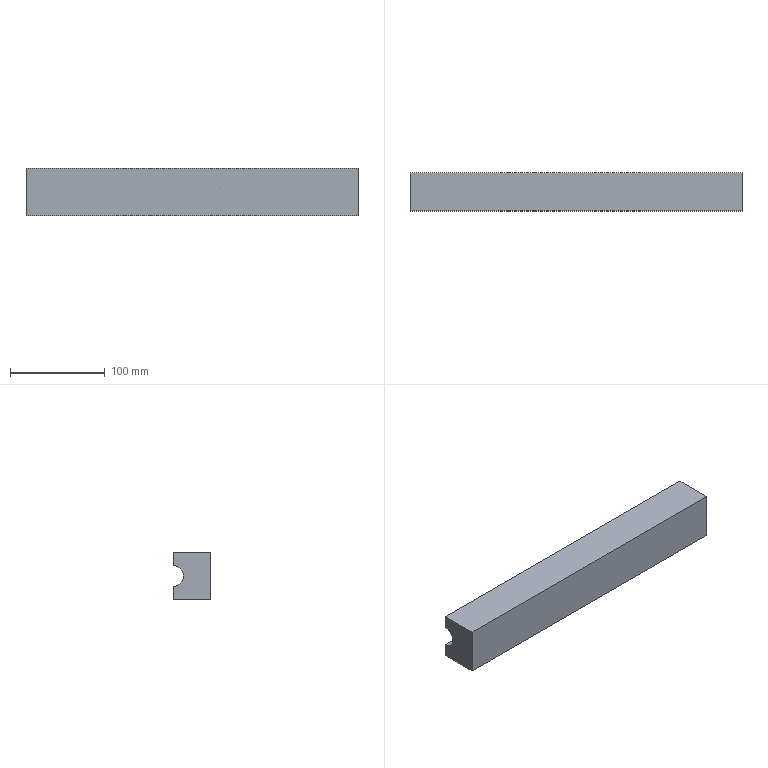Part | NX | features upper clamp 2 | 1 solid | 8 faces | box 350 x 40 x 50 mm | volume 632262 mm3 | plane 7 | cylinder 1 | commonest cylinder face diameters 22.2 x1
STEP:
#1=CARTESIAN_POINT('',(0.,0.,-11.1));
#2=VERTEX_POINT('',#1);
#3=CARTESIAN_POINT('',(0.,0.,11.1));
#4=VERTEX_POINT('',#3);
#5=CARTESIAN_POINT('',(0.,0.,0.));
#6=DIRECTION('',(1.,0.,0.));
#7=DIRECTION('',(0.,1.,0.));
#8=AXIS2_PLACEMENT_3D('',#5,#6,#7);
#9=CIRCLE('',#8,11.1);
#10=EDGE_CURVE('',#2,#4,#9,.F.);
#11=ORIENTED_EDGE('',*,*,#10,.F.);
#12=CARTESIAN_POINT('',(-350.,0.,-11.1));
#13=VERTEX_POINT('',#12);
#14=CARTESIAN_POINT('',(0.,0.,-11.1));
#15=DIRECTION('',(-1.,0.,0.));
#16=VECTOR('',#15,1000.);
#17=LINE('',#14,#16);
#18=EDGE_CURVE('',#13,#2,#17,.F.);
#19=ORIENTED_EDGE('',*,*,#18,.F.);
#20=CARTESIAN_POINT('',(-350.,0.,11.1));
#21=VERTEX_POINT('',#20);
#22=CARTESIAN_POINT('',(-350.,0.,0.));
#23=DIRECTION('',(1.,0.,0.));
#24=DIRECTION('',(0.,1.,0.));
#25=AXIS2_PLACEMENT_3D('',#22,#23,#24);
#26=CIRCLE('',#25,11.1);
#27=EDGE_CURVE('',#21,#13,#26,.T.);
#28=ORIENTED_EDGE('',*,*,#27,.F.);
#29=CARTESIAN_POINT('',(0.,0.,11.1));
#30=DIRECTION('',(-1.,0.,0.));
#31=VECTOR('',#30,1000.);
#32=LINE('',#29,#31);
#33=EDGE_CURVE('',#4,#21,#32,.T.);
#34=ORIENTED_EDGE('',*,*,#33,.F.);
#35=EDGE_LOOP('',(#11,#19,#28,#34));
#36=FACE_BOUND('',#35,.T.);
#37=CARTESIAN_POINT('',(-350.,0.,0.));
#38=DIRECTION('',(1.,0.,0.));
#39=DIRECTION('',(0.,1.,0.));
#40=AXIS2_PLACEMENT_3D('',#37,#38,#39);
#41=CYLINDRICAL_SURFACE('',#40,11.1);
#42=ADVANCED_FACE('',(#36),#41,.F.);
#43=CARTESIAN_POINT('',(-350.,0.,25.));
#44=VERTEX_POINT('',#43);
#45=CARTESIAN_POINT('',(0.,0.,25.));
#46=VERTEX_POINT('',#45);
#47=CARTESIAN_POINT('',(0.,0.,25.));
#48=DIRECTION('',(-1.,0.,0.));
#49=VECTOR('',#48,1000.);
#50=LINE('',#47,#49);
#51=EDGE_CURVE('',#44,#46,#50,.F.);
#52=ORIENTED_EDGE('',*,*,#51,.T.);
#53=CARTESIAN_POINT('',(0.,0.,-25.));
#54=DIRECTION('',(0.,0.,-1.));
#55=VECTOR('',#54,1000.);
#56=LINE('',#53,#55);
#57=EDGE_CURVE('',#4,#46,#56,.F.);
#58=ORIENTED_EDGE('',*,*,#57,.F.);
#59=ORIENTED_EDGE('',*,*,#33,.T.);
#60=CARTESIAN_POINT('',(-350.,0.,-25.));
#61=DIRECTION('',(0.,0.,1.));
#62=VECTOR('',#61,1000.);
#63=LINE('',#60,#62);
#64=EDGE_CURVE('',#44,#21,#63,.F.);
#65=ORIENTED_EDGE('',*,*,#64,.F.);
#66=EDGE_LOOP('',(#52,#58,#59,#65));
#67=FACE_BOUND('',#66,.T.);
#68=CARTESIAN_POINT('',(0.,0.,-25.));
#69=DIRECTION('',(0.,1.,0.));
#70=DIRECTION('',(-1.,0.,0.));
#71=AXIS2_PLACEMENT_3D('',#68,#69,#70);
#72=PLANE('',#71);
#73=ADVANCED_FACE('',(#67),#72,.T.);
#74=CARTESIAN_POINT('',(-350.,0.,-25.));
#75=VERTEX_POINT('',#74);
#76=CARTESIAN_POINT('',(0.,0.,-25.));
#77=VERTEX_POINT('',#76);
#78=CARTESIAN_POINT('',(0.,0.,-25.));
#79=DIRECTION('',(-1.,0.,0.));
#80=VECTOR('',#79,1000.);
#81=LINE('',#78,#80);
#82=EDGE_CURVE('',#75,#77,#81,.F.);
#83=ORIENTED_EDGE('',*,*,#82,.F.);
#84=CARTESIAN_POINT('',(-350.,0.,-25.));
#85=DIRECTION('',(0.,0.,1.));
#86=VECTOR('',#85,1000.);
#87=LINE('',#84,#86);
#88=EDGE_CURVE('',#13,#75,#87,.F.);
#89=ORIENTED_EDGE('',*,*,#88,.F.);
#90=ORIENTED_EDGE('',*,*,#18,.T.);
#91=CARTESIAN_POINT('',(0.,0.,-25.));
#92=DIRECTION('',(0.,0.,-1.));
#93=VECTOR('',#92,1000.);
#94=LINE('',#91,#93);
#95=EDGE_CURVE('',#77,#2,#94,.F.);
#96=ORIENTED_EDGE('',*,*,#95,.F.);
#97=EDGE_LOOP('',(#83,#89,#90,#96));
#98=FACE_BOUND('',#97,.T.);
#99=CARTESIAN_POINT('',(0.,0.,-25.));
#100=DIRECTION('',(0.,1.,0.));
#101=DIRECTION('',(-1.,0.,0.));
#102=AXIS2_PLACEMENT_3D('',#99,#100,#101);
#103=PLANE('',#102);
#104=ADVANCED_FACE('',(#98),#103,.T.);
#105=ORIENTED_EDGE('',*,*,#51,.F.);
#106=CARTESIAN_POINT('',(-350.,-40.,25.));
#107=VERTEX_POINT('',#106);
#108=CARTESIAN_POINT('',(-350.,0.,25.));
#109=DIRECTION('',(0.,1.,0.));
#110=VECTOR('',#109,1000.);
#111=LINE('',#108,#110);
#112=EDGE_CURVE('',#107,#44,#111,.T.);
#113=ORIENTED_EDGE('',*,*,#112,.F.);
#114=CARTESIAN_POINT('',(0.,-40.,25.));
#115=VERTEX_POINT('',#114);
#116=CARTESIAN_POINT('',(0.,-40.,25.));
#117=DIRECTION('',(1.,0.,0.));
#118=VECTOR('',#117,1000.);
#119=LINE('',#116,#118);
#120=EDGE_CURVE('',#115,#107,#119,.F.);
#121=ORIENTED_EDGE('',*,*,#120,.F.);
#122=CARTESIAN_POINT('',(0.,0.,25.));
#123=DIRECTION('',(0.,1.,0.));
#124=VECTOR('',#123,1000.);
#125=LINE('',#122,#124);
#126=EDGE_CURVE('',#46,#115,#125,.F.);
#127=ORIENTED_EDGE('',*,*,#126,.F.);
#128=EDGE_LOOP('',(#105,#113,#121,#127));
#129=FACE_BOUND('',#128,.T.);
#130=CARTESIAN_POINT('',(0.,-40.,25.));
#131=DIRECTION('',(0.,0.,-1.));
#132=DIRECTION('',(-1.,0.,0.));
#133=AXIS2_PLACEMENT_3D('',#130,#131,#132);
#134=PLANE('',#133);
#135=ADVANCED_FACE('',(#129),#134,.F.);
#136=ORIENTED_EDGE('',*,*,#112,.T.);
#137=ORIENTED_EDGE('',*,*,#64,.T.);
#138=ORIENTED_EDGE('',*,*,#27,.T.);
#139=ORIENTED_EDGE('',*,*,#88,.T.);
#140=CARTESIAN_POINT('',(-350.,-40.,-25.));
#141=VERTEX_POINT('',#140);
#142=CARTESIAN_POINT('',(-350.,-40.,-25.));
#143=DIRECTION('',(0.,1.,0.));
#144=VECTOR('',#143,1000.);
#145=LINE('',#142,#144);
#146=EDGE_CURVE('',#141,#75,#145,.T.);
#147=ORIENTED_EDGE('',*,*,#146,.F.);
#148=CARTESIAN_POINT('',(-350.,-40.,-25.));
#149=DIRECTION('',(0.,0.,1.));
#150=VECTOR('',#149,1000.);
#151=LINE('',#148,#150);
#152=EDGE_CURVE('',#107,#141,#151,.F.);
#153=ORIENTED_EDGE('',*,*,#152,.F.);
#154=EDGE_LOOP('',(#136,#137,#138,#139,#147,#153));
#155=FACE_BOUND('',#154,.T.);
#156=CARTESIAN_POINT('',(-350.,0.,-25.));
#157=DIRECTION('',(-1.,0.,0.));
#158=DIRECTION('',(0.,0.,1.));
#159=AXIS2_PLACEMENT_3D('',#156,#157,#158);
#160=PLANE('',#159);
#161=ADVANCED_FACE('',(#155),#160,.T.);
#162=ORIENTED_EDGE('',*,*,#146,.T.);
#163=ORIENTED_EDGE('',*,*,#82,.T.);
#164=CARTESIAN_POINT('',(0.,-40.,-25.));
#165=VERTEX_POINT('',#164);
#166=CARTESIAN_POINT('',(0.,0.,-25.));
#167=DIRECTION('',(0.,1.,0.));
#168=VECTOR('',#167,1000.);
#169=LINE('',#166,#168);
#170=EDGE_CURVE('',#165,#77,#169,.T.);
#171=ORIENTED_EDGE('',*,*,#170,.F.);
#172=CARTESIAN_POINT('',(0.,-40.,-25.));
#173=DIRECTION('',(1.,0.,0.));
#174=VECTOR('',#173,1000.);
#175=LINE('',#172,#174);
#176=EDGE_CURVE('',#141,#165,#175,.T.);
#177=ORIENTED_EDGE('',*,*,#176,.F.);
#178=EDGE_LOOP('',(#162,#163,#171,#177));
#179=FACE_BOUND('',#178,.T.);
#180=CARTESIAN_POINT('',(0.,-40.,-25.));
#181=DIRECTION('',(0.,0.,-1.));
#182=DIRECTION('',(-1.,0.,0.));
#183=AXIS2_PLACEMENT_3D('',#180,#181,#182);
#184=PLANE('',#183);
#185=ADVANCED_FACE('',(#179),#184,.T.);
#186=ORIENTED_EDGE('',*,*,#170,.T.);
#187=ORIENTED_EDGE('',*,*,#95,.T.);
#188=ORIENTED_EDGE('',*,*,#10,.T.);
#189=ORIENTED_EDGE('',*,*,#57,.T.);
#190=ORIENTED_EDGE('',*,*,#126,.T.);
#191=CARTESIAN_POINT('',(0.,-40.,-25.));
#192=DIRECTION('',(0.,0.,1.));
#193=VECTOR('',#192,1000.);
#194=LINE('',#191,#193);
#195=EDGE_CURVE('',#165,#115,#194,.T.);
#196=ORIENTED_EDGE('',*,*,#195,.F.);
#197=EDGE_LOOP('',(#186,#187,#188,#189,#190,#196));
#198=FACE_BOUND('',#197,.T.);
#199=CARTESIAN_POINT('',(0.,0.,-25.));
#200=DIRECTION('',(1.,0.,0.));
#201=DIRECTION('',(0.,0.,-1.));
#202=AXIS2_PLACEMENT_3D('',#199,#200,#201);
#203=PLANE('',#202);
#204=ADVANCED_FACE('',(#198),#203,.T.);
#205=ORIENTED_EDGE('',*,*,#176,.T.);
#206=ORIENTED_EDGE('',*,*,#195,.T.);
#207=ORIENTED_EDGE('',*,*,#120,.T.);
#208=ORIENTED_EDGE('',*,*,#152,.T.);
#209=EDGE_LOOP('',(#205,#206,#207,#208));
#210=FACE_BOUND('',#209,.T.);
#211=CARTESIAN_POINT('',(0.,-40.,-25.));
#212=DIRECTION('',(0.,-1.,0.));
#213=DIRECTION('',(1.,0.,0.));
#214=AXIS2_PLACEMENT_3D('',#211,#212,#213);
#215=PLANE('',#214);
#216=ADVANCED_FACE('',(#210),#215,.T.);
#217=CLOSED_SHELL('',(#42,#73,#104,#135,#161,#185,#204,#216));
#218=MANIFOLD_SOLID_BREP('',#217);
#219=(LENGTH_UNIT()NAMED_UNIT(*)SI_UNIT(.MILLI.,.METRE.));
#220=UNCERTAINTY_MEASURE_WITH_UNIT(LENGTH_MEASURE(0.00001),#219,'','');
#221=(NAMED_UNIT(*)PLANE_ANGLE_UNIT()SI_UNIT($,.RADIAN.));
#222=(NAMED_UNIT(*)SI_UNIT($,.STERADIAN.)SOLID_ANGLE_UNIT());
#223=(GEOMETRIC_REPRESENTATION_CONTEXT(3)GLOBAL_UNCERTAINTY_ASSIGNED_CONTEXT((#220))GLOBAL_UNIT_ASSIGNED_CONTEXT((#219,#221,#222))REPRESENTATION_CONTEXT('',''));
#224=ADVANCED_BREP_SHAPE_REPRESENTATION('',(#218),#223);